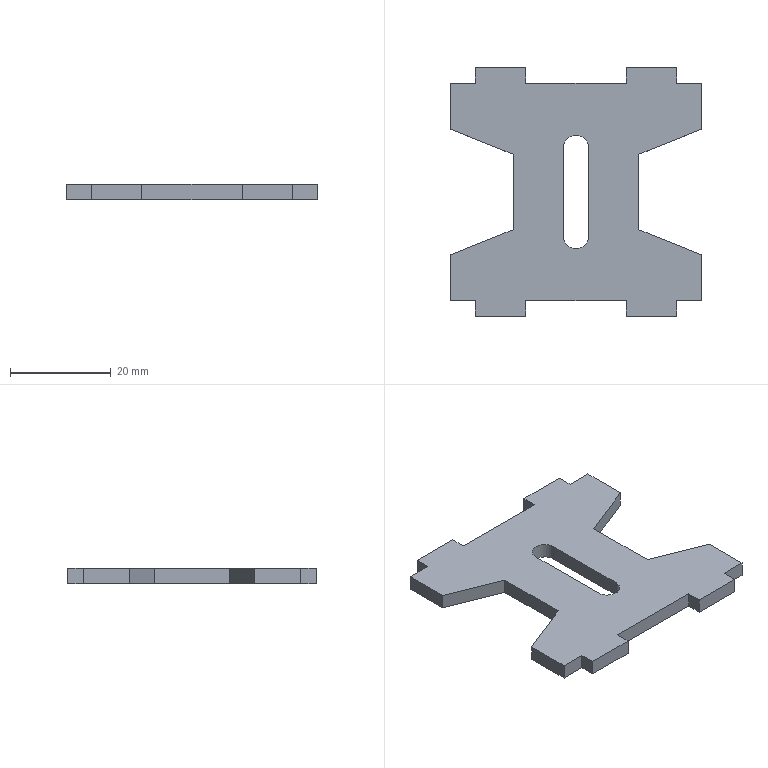Part | SolidWorks | features Extrusion 1 | 1 solid | 34 faces | box 50 x 49.3 x 3 mm | volume 5034 mm3 | plane 32 | cylinder 2 | commonest cylinder face diameters 5 x2
STEP:
#1=CARTESIAN_POINT('',(-25.609,-21.769,3.));
#2=VERTEX_POINT('',#1);
#3=CARTESIAN_POINT('',(-25.609,-12.619,3.));
#4=VERTEX_POINT('',#3);
#5=CARTESIAN_POINT('',(-25.609,-21.769,3.));
#6=DIRECTION('',(0.,1.,0.));
#7=VECTOR('',#6,1000.);
#8=LINE('',#5,#7);
#9=EDGE_CURVE('',#2,#4,#8,.T.);
#10=ORIENTED_EDGE('',*,*,#9,.F.);
#11=CARTESIAN_POINT('',(-20.609,-21.769,3.));
#12=VERTEX_POINT('',#11);
#13=CARTESIAN_POINT('',(-25.609,-21.769,3.));
#14=DIRECTION('',(1.,0.,0.));
#15=VECTOR('',#14,1000.);
#16=LINE('',#13,#15);
#17=EDGE_CURVE('',#2,#12,#16,.T.);
#18=ORIENTED_EDGE('',*,*,#17,.T.);
#19=CARTESIAN_POINT('',(-20.609,-24.769,3.));
#20=VERTEX_POINT('',#19);
#21=CARTESIAN_POINT('',(-20.609,-21.769,3.));
#22=DIRECTION('',(0.,-1.,0.));
#23=VECTOR('',#22,1000.);
#24=LINE('',#21,#23);
#25=EDGE_CURVE('',#12,#20,#24,.T.);
#26=ORIENTED_EDGE('',*,*,#25,.T.);
#27=CARTESIAN_POINT('',(-10.609,-24.769,3.));
#28=VERTEX_POINT('',#27);
#29=CARTESIAN_POINT('',(-20.609,-24.769,3.));
#30=DIRECTION('',(1.,0.,0.));
#31=VECTOR('',#30,1000.);
#32=LINE('',#29,#31);
#33=EDGE_CURVE('',#20,#28,#32,.T.);
#34=ORIENTED_EDGE('',*,*,#33,.T.);
#35=CARTESIAN_POINT('',(-10.609,-21.769,3.));
#36=VERTEX_POINT('',#35);
#37=CARTESIAN_POINT('',(-10.609,-24.769,3.));
#38=DIRECTION('',(0.,1.,0.));
#39=VECTOR('',#38,1000.);
#40=LINE('',#37,#39);
#41=EDGE_CURVE('',#28,#36,#40,.T.);
#42=ORIENTED_EDGE('',*,*,#41,.T.);
#43=CARTESIAN_POINT('',(9.391,-21.769,3.));
#44=VERTEX_POINT('',#43);
#45=CARTESIAN_POINT('',(-10.609,-21.769,3.));
#46=DIRECTION('',(1.,0.,0.));
#47=VECTOR('',#46,1000.);
#48=LINE('',#45,#47);
#49=EDGE_CURVE('',#36,#44,#48,.T.);
#50=ORIENTED_EDGE('',*,*,#49,.T.);
#51=CARTESIAN_POINT('',(9.391,-24.769,3.));
#52=VERTEX_POINT('',#51);
#53=CARTESIAN_POINT('',(9.391,-24.769,3.));
#54=DIRECTION('',(0.,1.,0.));
#55=VECTOR('',#54,1000.);
#56=LINE('',#53,#55);
#57=EDGE_CURVE('',#52,#44,#56,.T.);
#58=ORIENTED_EDGE('',*,*,#57,.F.);
#59=CARTESIAN_POINT('',(19.391,-24.769,3.));
#60=VERTEX_POINT('',#59);
#61=CARTESIAN_POINT('',(19.391,-24.769,3.));
#62=DIRECTION('',(-1.,0.,0.));
#63=VECTOR('',#62,1000.);
#64=LINE('',#61,#63);
#65=EDGE_CURVE('',#60,#52,#64,.T.);
#66=ORIENTED_EDGE('',*,*,#65,.F.);
#67=CARTESIAN_POINT('',(19.391,-21.769,3.));
#68=VERTEX_POINT('',#67);
#69=CARTESIAN_POINT('',(19.391,-21.769,3.));
#70=DIRECTION('',(0.,-1.,0.));
#71=VECTOR('',#70,1000.);
#72=LINE('',#69,#71);
#73=EDGE_CURVE('',#68,#60,#72,.T.);
#74=ORIENTED_EDGE('',*,*,#73,.F.);
#75=CARTESIAN_POINT('',(24.391,-21.769,3.));
#76=VERTEX_POINT('',#75);
#77=CARTESIAN_POINT('',(19.391,-21.769,3.));
#78=DIRECTION('',(1.,0.,0.));
#79=VECTOR('',#78,1000.);
#80=LINE('',#77,#79);
#81=EDGE_CURVE('',#68,#76,#80,.T.);
#82=ORIENTED_EDGE('',*,*,#81,.T.);
#83=CARTESIAN_POINT('',(24.391,-12.619,3.));
#84=VERTEX_POINT('',#83);
#85=CARTESIAN_POINT('',(24.391,-21.769,3.));
#86=DIRECTION('',(0.,1.,0.));
#87=VECTOR('',#86,1000.);
#88=LINE('',#85,#87);
#89=EDGE_CURVE('',#76,#84,#88,.T.);
#90=ORIENTED_EDGE('',*,*,#89,.T.);
#91=CARTESIAN_POINT('',(11.891,-7.619,3.));
#92=VERTEX_POINT('',#91);
#93=CARTESIAN_POINT('',(11.891,-7.619,3.));
#94=DIRECTION('',(0.9285,-0.3714,0.));
#95=VECTOR('',#94,1000.);
#96=LINE('',#93,#95);
#97=EDGE_CURVE('',#92,#84,#96,.T.);
#98=ORIENTED_EDGE('',*,*,#97,.F.);
#99=CARTESIAN_POINT('',(11.891,7.381,3.));
#100=VERTEX_POINT('',#99);
#101=CARTESIAN_POINT('',(11.891,7.381,3.));
#102=DIRECTION('',(0.,-1.,0.));
#103=VECTOR('',#102,1000.);
#104=LINE('',#101,#103);
#105=EDGE_CURVE('',#100,#92,#104,.T.);
#106=ORIENTED_EDGE('',*,*,#105,.F.);
#107=CARTESIAN_POINT('',(24.391,12.381,3.));
#108=VERTEX_POINT('',#107);
#109=CARTESIAN_POINT('',(24.391,12.381,3.));
#110=DIRECTION('',(-0.9285,-0.3714,0.));
#111=VECTOR('',#110,1000.);
#112=LINE('',#109,#111);
#113=EDGE_CURVE('',#108,#100,#112,.T.);
#114=ORIENTED_EDGE('',*,*,#113,.F.);
#115=CARTESIAN_POINT('',(24.391,21.531,3.));
#116=VERTEX_POINT('',#115);
#117=CARTESIAN_POINT('',(24.391,12.381,3.));
#118=DIRECTION('',(0.,1.,0.));
#119=VECTOR('',#118,1000.);
#120=LINE('',#117,#119);
#121=EDGE_CURVE('',#108,#116,#120,.T.);
#122=ORIENTED_EDGE('',*,*,#121,.T.);
#123=CARTESIAN_POINT('',(19.391,21.531,3.));
#124=VERTEX_POINT('',#123);
#125=CARTESIAN_POINT('',(19.391,21.531,3.));
#126=DIRECTION('',(1.,0.,0.));
#127=VECTOR('',#126,1000.);
#128=LINE('',#125,#127);
#129=EDGE_CURVE('',#124,#116,#128,.T.);
#130=ORIENTED_EDGE('',*,*,#129,.F.);
#131=CARTESIAN_POINT('',(19.391,24.531,3.));
#132=VERTEX_POINT('',#131);
#133=CARTESIAN_POINT('',(19.391,21.531,3.));
#134=DIRECTION('',(0.,1.,0.));
#135=VECTOR('',#134,1000.);
#136=LINE('',#133,#135);
#137=EDGE_CURVE('',#124,#132,#136,.T.);
#138=ORIENTED_EDGE('',*,*,#137,.T.);
#139=CARTESIAN_POINT('',(9.391,24.531,3.));
#140=VERTEX_POINT('',#139);
#141=CARTESIAN_POINT('',(19.391,24.531,3.));
#142=DIRECTION('',(-1.,0.,0.));
#143=VECTOR('',#142,1000.);
#144=LINE('',#141,#143);
#145=EDGE_CURVE('',#132,#140,#144,.T.);
#146=ORIENTED_EDGE('',*,*,#145,.T.);
#147=CARTESIAN_POINT('',(9.391,21.531,3.));
#148=VERTEX_POINT('',#147);
#149=CARTESIAN_POINT('',(9.391,24.531,3.));
#150=DIRECTION('',(0.,-1.,0.));
#151=VECTOR('',#150,1000.);
#152=LINE('',#149,#151);
#153=EDGE_CURVE('',#140,#148,#152,.T.);
#154=ORIENTED_EDGE('',*,*,#153,.T.);
#155=CARTESIAN_POINT('',(-10.609,21.531,3.));
#156=VERTEX_POINT('',#155);
#157=CARTESIAN_POINT('',(-10.609,21.531,3.));
#158=DIRECTION('',(1.,0.,0.));
#159=VECTOR('',#158,1000.);
#160=LINE('',#157,#159);
#161=EDGE_CURVE('',#156,#148,#160,.T.);
#162=ORIENTED_EDGE('',*,*,#161,.F.);
#163=CARTESIAN_POINT('',(-10.609,24.531,3.));
#164=VERTEX_POINT('',#163);
#165=CARTESIAN_POINT('',(-10.609,24.531,3.));
#166=DIRECTION('',(0.,-1.,0.));
#167=VECTOR('',#166,1000.);
#168=LINE('',#165,#167);
#169=EDGE_CURVE('',#164,#156,#168,.T.);
#170=ORIENTED_EDGE('',*,*,#169,.F.);
#171=CARTESIAN_POINT('',(-20.609,24.531,3.));
#172=VERTEX_POINT('',#171);
#173=CARTESIAN_POINT('',(-20.609,24.531,3.));
#174=DIRECTION('',(1.,0.,0.));
#175=VECTOR('',#174,1000.);
#176=LINE('',#173,#175);
#177=EDGE_CURVE('',#172,#164,#176,.T.);
#178=ORIENTED_EDGE('',*,*,#177,.F.);
#179=CARTESIAN_POINT('',(-20.609,21.531,3.));
#180=VERTEX_POINT('',#179);
#181=CARTESIAN_POINT('',(-20.609,21.531,3.));
#182=DIRECTION('',(0.,1.,0.));
#183=VECTOR('',#182,1000.);
#184=LINE('',#181,#183);
#185=EDGE_CURVE('',#180,#172,#184,.T.);
#186=ORIENTED_EDGE('',*,*,#185,.F.);
#187=CARTESIAN_POINT('',(-25.609,21.531,3.));
#188=VERTEX_POINT('',#187);
#189=CARTESIAN_POINT('',(-25.609,21.531,3.));
#190=DIRECTION('',(1.,0.,0.));
#191=VECTOR('',#190,1000.);
#192=LINE('',#189,#191);
#193=EDGE_CURVE('',#188,#180,#192,.T.);
#194=ORIENTED_EDGE('',*,*,#193,.F.);
#195=CARTESIAN_POINT('',(-25.609,12.381,3.));
#196=VERTEX_POINT('',#195);
#197=CARTESIAN_POINT('',(-25.609,12.381,3.));
#198=DIRECTION('',(0.,1.,0.));
#199=VECTOR('',#198,1000.);
#200=LINE('',#197,#199);
#201=EDGE_CURVE('',#196,#188,#200,.T.);
#202=ORIENTED_EDGE('',*,*,#201,.F.);
#203=CARTESIAN_POINT('',(-13.109,7.381,3.));
#204=VERTEX_POINT('',#203);
#205=CARTESIAN_POINT('',(-25.609,12.381,3.));
#206=DIRECTION('',(0.9285,-0.3714,0.));
#207=VECTOR('',#206,1000.);
#208=LINE('',#205,#207);
#209=EDGE_CURVE('',#196,#204,#208,.T.);
#210=ORIENTED_EDGE('',*,*,#209,.T.);
#211=CARTESIAN_POINT('',(-13.109,-7.619,3.));
#212=VERTEX_POINT('',#211);
#213=CARTESIAN_POINT('',(-13.109,7.381,3.));
#214=DIRECTION('',(0.,-1.,0.));
#215=VECTOR('',#214,1000.);
#216=LINE('',#213,#215);
#217=EDGE_CURVE('',#204,#212,#216,.T.);
#218=ORIENTED_EDGE('',*,*,#217,.T.);
#219=CARTESIAN_POINT('',(-13.109,-7.619,3.));
#220=DIRECTION('',(-0.9285,-0.3714,0.));
#221=VECTOR('',#220,1000.);
#222=LINE('',#219,#221);
#223=EDGE_CURVE('',#212,#4,#222,.T.);
#224=ORIENTED_EDGE('',*,*,#223,.T.);
#225=EDGE_LOOP('',(#10,#18,#26,#34,#42,#50,#58,#66,#74,#82,#90,#98,#106,#114,#122,#130,#138,#146,#154,#162,#170,#178,#186,#194,#202,#210,#218,#224));
#226=FACE_OUTER_BOUND('',#225,.T.);
#227=CARTESIAN_POINT('',(1.891,8.631,3.));
#228=VERTEX_POINT('',#227);
#229=CARTESIAN_POINT('',(-3.109,8.631,3.));
#230=VERTEX_POINT('',#229);
#231=CARTESIAN_POINT('',(-0.6092,8.631,3.));
#232=DIRECTION('',(0.,0.,1.));
#233=DIRECTION('',(1.,0.,0.));
#234=AXIS2_PLACEMENT_3D('',#231,#232,#233);
#235=CIRCLE('',#234,2.5);
#236=EDGE_CURVE('',#228,#230,#235,.T.);
#237=ORIENTED_EDGE('',*,*,#236,.F.);
#238=CARTESIAN_POINT('',(1.891,-8.869,3.));
#239=VERTEX_POINT('',#238);
#240=CARTESIAN_POINT('',(1.891,8.631,3.));
#241=DIRECTION('',(0.,-1.,0.));
#242=VECTOR('',#241,1000.);
#243=LINE('',#240,#242);
#244=EDGE_CURVE('',#228,#239,#243,.T.);
#245=ORIENTED_EDGE('',*,*,#244,.T.);
#246=CARTESIAN_POINT('',(-3.109,-8.869,3.));
#247=VERTEX_POINT('',#246);
#248=CARTESIAN_POINT('',(-0.6092,-8.869,3.));
#249=DIRECTION('',(0.,0.,1.));
#250=DIRECTION('',(1.,0.,0.));
#251=AXIS2_PLACEMENT_3D('',#248,#249,#250);
#252=CIRCLE('',#251,2.5);
#253=EDGE_CURVE('',#247,#239,#252,.T.);
#254=ORIENTED_EDGE('',*,*,#253,.F.);
#255=CARTESIAN_POINT('',(-3.109,8.631,3.));
#256=DIRECTION('',(0.,-1.,0.));
#257=VECTOR('',#256,1000.);
#258=LINE('',#255,#257);
#259=EDGE_CURVE('',#230,#247,#258,.T.);
#260=ORIENTED_EDGE('',*,*,#259,.F.);
#261=EDGE_LOOP('',(#237,#245,#254,#260));
#262=FACE_BOUND('',#261,.T.);
#263=CARTESIAN_POINT('',(0.,0.,3.));
#264=DIRECTION('',(0.,0.,-1.));
#265=DIRECTION('',(-1.,0.,0.));
#266=AXIS2_PLACEMENT_3D('',#263,#264,#265);
#267=PLANE('',#266);
#268=ADVANCED_FACE('',(#226,#262),#267,.F.);
#269=CARTESIAN_POINT('',(-25.609,-21.769,0.));
#270=VERTEX_POINT('',#269);
#271=CARTESIAN_POINT('',(-25.609,-12.619,0.));
#272=VERTEX_POINT('',#271);
#273=CARTESIAN_POINT('',(-25.609,-21.769,0.));
#274=DIRECTION('',(0.,1.,0.));
#275=VECTOR('',#274,1000.);
#276=LINE('',#273,#275);
#277=EDGE_CURVE('',#270,#272,#276,.T.);
#278=ORIENTED_EDGE('',*,*,#277,.T.);
#279=CARTESIAN_POINT('',(-13.109,-7.619,0.));
#280=VERTEX_POINT('',#279);
#281=CARTESIAN_POINT('',(-13.109,-7.619,0.));
#282=DIRECTION('',(-0.9285,-0.3714,0.));
#283=VECTOR('',#282,1000.);
#284=LINE('',#281,#283);
#285=EDGE_CURVE('',#280,#272,#284,.T.);
#286=ORIENTED_EDGE('',*,*,#285,.F.);
#287=CARTESIAN_POINT('',(-13.109,7.381,0.));
#288=VERTEX_POINT('',#287);
#289=CARTESIAN_POINT('',(-13.109,7.381,0.));
#290=DIRECTION('',(0.,-1.,0.));
#291=VECTOR('',#290,1000.);
#292=LINE('',#289,#291);
#293=EDGE_CURVE('',#288,#280,#292,.T.);
#294=ORIENTED_EDGE('',*,*,#293,.F.);
#295=CARTESIAN_POINT('',(-25.609,12.381,0.));
#296=VERTEX_POINT('',#295);
#297=CARTESIAN_POINT('',(-25.609,12.381,0.));
#298=DIRECTION('',(0.9285,-0.3714,0.));
#299=VECTOR('',#298,1000.);
#300=LINE('',#297,#299);
#301=EDGE_CURVE('',#296,#288,#300,.T.);
#302=ORIENTED_EDGE('',*,*,#301,.F.);
#303=CARTESIAN_POINT('',(-25.609,21.531,0.));
#304=VERTEX_POINT('',#303);
#305=CARTESIAN_POINT('',(-25.609,12.381,0.));
#306=DIRECTION('',(0.,1.,0.));
#307=VECTOR('',#306,1000.);
#308=LINE('',#305,#307);
#309=EDGE_CURVE('',#296,#304,#308,.T.);
#310=ORIENTED_EDGE('',*,*,#309,.T.);
#311=CARTESIAN_POINT('',(-20.609,21.531,0.));
#312=VERTEX_POINT('',#311);
#313=CARTESIAN_POINT('',(-25.609,21.531,0.));
#314=DIRECTION('',(1.,0.,0.));
#315=VECTOR('',#314,1000.);
#316=LINE('',#313,#315);
#317=EDGE_CURVE('',#304,#312,#316,.T.);
#318=ORIENTED_EDGE('',*,*,#317,.T.);
#319=CARTESIAN_POINT('',(-20.609,24.531,0.));
#320=VERTEX_POINT('',#319);
#321=CARTESIAN_POINT('',(-20.609,21.531,0.));
#322=DIRECTION('',(0.,1.,0.));
#323=VECTOR('',#322,1000.);
#324=LINE('',#321,#323);
#325=EDGE_CURVE('',#312,#320,#324,.T.);
#326=ORIENTED_EDGE('',*,*,#325,.T.);
#327=CARTESIAN_POINT('',(-10.609,24.531,0.));
#328=VERTEX_POINT('',#327);
#329=CARTESIAN_POINT('',(-20.609,24.531,0.));
#330=DIRECTION('',(1.,0.,0.));
#331=VECTOR('',#330,1000.);
#332=LINE('',#329,#331);
#333=EDGE_CURVE('',#320,#328,#332,.T.);
#334=ORIENTED_EDGE('',*,*,#333,.T.);
#335=CARTESIAN_POINT('',(-10.609,21.531,0.));
#336=VERTEX_POINT('',#335);
#337=CARTESIAN_POINT('',(-10.609,24.531,0.));
#338=DIRECTION('',(0.,-1.,0.));
#339=VECTOR('',#338,1000.);
#340=LINE('',#337,#339);
#341=EDGE_CURVE('',#328,#336,#340,.T.);
#342=ORIENTED_EDGE('',*,*,#341,.T.);
#343=CARTESIAN_POINT('',(9.391,21.531,0.));
#344=VERTEX_POINT('',#343);
#345=CARTESIAN_POINT('',(-10.609,21.531,0.));
#346=DIRECTION('',(1.,0.,0.));
#347=VECTOR('',#346,1000.);
#348=LINE('',#345,#347);
#349=EDGE_CURVE('',#336,#344,#348,.T.);
#350=ORIENTED_EDGE('',*,*,#349,.T.);
#351=CARTESIAN_POINT('',(9.391,24.531,0.));
#352=VERTEX_POINT('',#351);
#353=CARTESIAN_POINT('',(9.391,24.531,0.));
#354=DIRECTION('',(0.,-1.,0.));
#355=VECTOR('',#354,1000.);
#356=LINE('',#353,#355);
#357=EDGE_CURVE('',#352,#344,#356,.T.);
#358=ORIENTED_EDGE('',*,*,#357,.F.);
#359=CARTESIAN_POINT('',(19.391,24.531,0.));
#360=VERTEX_POINT('',#359);
#361=CARTESIAN_POINT('',(19.391,24.531,0.));
#362=DIRECTION('',(-1.,0.,0.));
#363=VECTOR('',#362,1000.);
#364=LINE('',#361,#363);
#365=EDGE_CURVE('',#360,#352,#364,.T.);
#366=ORIENTED_EDGE('',*,*,#365,.F.);
#367=CARTESIAN_POINT('',(19.391,21.531,0.));
#368=VERTEX_POINT('',#367);
#369=CARTESIAN_POINT('',(19.391,21.531,0.));
#370=DIRECTION('',(0.,1.,0.));
#371=VECTOR('',#370,1000.);
#372=LINE('',#369,#371);
#373=EDGE_CURVE('',#368,#360,#372,.T.);
#374=ORIENTED_EDGE('',*,*,#373,.F.);
#375=CARTESIAN_POINT('',(24.391,21.531,0.));
#376=VERTEX_POINT('',#375);
#377=CARTESIAN_POINT('',(19.391,21.531,0.));
#378=DIRECTION('',(1.,0.,0.));
#379=VECTOR('',#378,1000.);
#380=LINE('',#377,#379);
#381=EDGE_CURVE('',#368,#376,#380,.T.);
#382=ORIENTED_EDGE('',*,*,#381,.T.);
#383=CARTESIAN_POINT('',(24.391,12.381,0.));
#384=VERTEX_POINT('',#383);
#385=CARTESIAN_POINT('',(24.391,12.381,0.));
#386=DIRECTION('',(0.,1.,0.));
#387=VECTOR('',#386,1000.);
#388=LINE('',#385,#387);
#389=EDGE_CURVE('',#384,#376,#388,.T.);
#390=ORIENTED_EDGE('',*,*,#389,.F.);
#391=CARTESIAN_POINT('',(11.891,7.381,0.));
#392=VERTEX_POINT('',#391);
#393=CARTESIAN_POINT('',(24.391,12.381,0.));
#394=DIRECTION('',(-0.9285,-0.3714,0.));
#395=VECTOR('',#394,1000.);
#396=LINE('',#393,#395);
#397=EDGE_CURVE('',#384,#392,#396,.T.);
#398=ORIENTED_EDGE('',*,*,#397,.T.);
#399=CARTESIAN_POINT('',(11.891,-7.619,0.));
#400=VERTEX_POINT('',#399);
#401=CARTESIAN_POINT('',(11.891,7.381,0.));
#402=DIRECTION('',(0.,-1.,0.));
#403=VECTOR('',#402,1000.);
#404=LINE('',#401,#403);
#405=EDGE_CURVE('',#392,#400,#404,.T.);
#406=ORIENTED_EDGE('',*,*,#405,.T.);
#407=CARTESIAN_POINT('',(24.391,-12.619,0.));
#408=VERTEX_POINT('',#407);
#409=CARTESIAN_POINT('',(11.891,-7.619,0.));
#410=DIRECTION('',(0.9285,-0.3714,0.));
#411=VECTOR('',#410,1000.);
#412=LINE('',#409,#411);
#413=EDGE_CURVE('',#400,#408,#412,.T.);
#414=ORIENTED_EDGE('',*,*,#413,.T.);
#415=CARTESIAN_POINT('',(24.391,-21.769,0.));
#416=VERTEX_POINT('',#415);
#417=CARTESIAN_POINT('',(24.391,-21.769,0.));
#418=DIRECTION('',(0.,1.,0.));
#419=VECTOR('',#418,1000.);
#420=LINE('',#417,#419);
#421=EDGE_CURVE('',#416,#408,#420,.T.);
#422=ORIENTED_EDGE('',*,*,#421,.F.);
#423=CARTESIAN_POINT('',(19.391,-21.769,0.));
#424=VERTEX_POINT('',#423);
#425=CARTESIAN_POINT('',(19.391,-21.769,0.));
#426=DIRECTION('',(1.,0.,0.));
#427=VECTOR('',#426,1000.);
#428=LINE('',#425,#427);
#429=EDGE_CURVE('',#424,#416,#428,.T.);
#430=ORIENTED_EDGE('',*,*,#429,.F.);
#431=CARTESIAN_POINT('',(19.391,-24.769,0.));
#432=VERTEX_POINT('',#431);
#433=CARTESIAN_POINT('',(19.391,-21.769,0.));
#434=DIRECTION('',(0.,-1.,0.));
#435=VECTOR('',#434,1000.);
#436=LINE('',#433,#435);
#437=EDGE_CURVE('',#424,#432,#436,.T.);
#438=ORIENTED_EDGE('',*,*,#437,.T.);
#439=CARTESIAN_POINT('',(9.391,-24.769,0.));
#440=VERTEX_POINT('',#439);
#441=CARTESIAN_POINT('',(19.391,-24.769,0.));
#442=DIRECTION('',(-1.,0.,0.));
#443=VECTOR('',#442,1000.);
#444=LINE('',#441,#443);
#445=EDGE_CURVE('',#432,#440,#444,.T.);
#446=ORIENTED_EDGE('',*,*,#445,.T.);
#447=CARTESIAN_POINT('',(9.391,-21.769,0.));
#448=VERTEX_POINT('',#447);
#449=CARTESIAN_POINT('',(9.391,-24.769,0.));
#450=DIRECTION('',(0.,1.,0.));
#451=VECTOR('',#450,1000.);
#452=LINE('',#449,#451);
#453=EDGE_CURVE('',#440,#448,#452,.T.);
#454=ORIENTED_EDGE('',*,*,#453,.T.);
#455=CARTESIAN_POINT('',(-10.609,-21.769,0.));
#456=VERTEX_POINT('',#455);
#457=CARTESIAN_POINT('',(-10.609,-21.769,0.));
#458=DIRECTION('',(1.,0.,0.));
#459=VECTOR('',#458,1000.);
#460=LINE('',#457,#459);
#461=EDGE_CURVE('',#456,#448,#460,.T.);
#462=ORIENTED_EDGE('',*,*,#461,.F.);
#463=CARTESIAN_POINT('',(-10.609,-24.769,0.));
#464=VERTEX_POINT('',#463);
#465=CARTESIAN_POINT('',(-10.609,-24.769,0.));
#466=DIRECTION('',(0.,1.,0.));
#467=VECTOR('',#466,1000.);
#468=LINE('',#465,#467);
#469=EDGE_CURVE('',#464,#456,#468,.T.);
#470=ORIENTED_EDGE('',*,*,#469,.F.);
#471=CARTESIAN_POINT('',(-20.609,-24.769,0.));
#472=VERTEX_POINT('',#471);
#473=CARTESIAN_POINT('',(-20.609,-24.769,0.));
#474=DIRECTION('',(1.,0.,0.));
#475=VECTOR('',#474,1000.);
#476=LINE('',#473,#475);
#477=EDGE_CURVE('',#472,#464,#476,.T.);
#478=ORIENTED_EDGE('',*,*,#477,.F.);
#479=CARTESIAN_POINT('',(-20.609,-21.769,0.));
#480=VERTEX_POINT('',#479);
#481=CARTESIAN_POINT('',(-20.609,-21.769,0.));
#482=DIRECTION('',(0.,-1.,0.));
#483=VECTOR('',#482,1000.);
#484=LINE('',#481,#483);
#485=EDGE_CURVE('',#480,#472,#484,.T.);
#486=ORIENTED_EDGE('',*,*,#485,.F.);
#487=CARTESIAN_POINT('',(-25.609,-21.769,0.));
#488=DIRECTION('',(1.,0.,0.));
#489=VECTOR('',#488,1000.);
#490=LINE('',#487,#489);
#491=EDGE_CURVE('',#270,#480,#490,.T.);
#492=ORIENTED_EDGE('',*,*,#491,.F.);
#493=EDGE_LOOP('',(#278,#286,#294,#302,#310,#318,#326,#334,#342,#350,#358,#366,#374,#382,#390,#398,#406,#414,#422,#430,#438,#446,#454,#462,#470,#478,#486,#492));
#494=FACE_OUTER_BOUND('',#493,.T.);
#495=CARTESIAN_POINT('',(1.891,8.631,0.));
#496=VERTEX_POINT('',#495);
#497=CARTESIAN_POINT('',(1.891,-8.869,0.));
#498=VERTEX_POINT('',#497);
#499=CARTESIAN_POINT('',(1.891,8.631,0.));
#500=DIRECTION('',(0.,-1.,0.));
#501=VECTOR('',#500,1000.);
#502=LINE('',#499,#501);
#503=EDGE_CURVE('',#496,#498,#502,.T.);
#504=ORIENTED_EDGE('',*,*,#503,.F.);
#505=CARTESIAN_POINT('',(-3.109,8.631,0.));
#506=VERTEX_POINT('',#505);
#507=CARTESIAN_POINT('',(-0.6092,8.631,0.));
#508=DIRECTION('',(0.,0.,1.));
#509=DIRECTION('',(1.,0.,0.));
#510=AXIS2_PLACEMENT_3D('',#507,#508,#509);
#511=CIRCLE('',#510,2.5);
#512=EDGE_CURVE('',#496,#506,#511,.T.);
#513=ORIENTED_EDGE('',*,*,#512,.T.);
#514=CARTESIAN_POINT('',(-3.109,-8.869,0.));
#515=VERTEX_POINT('',#514);
#516=CARTESIAN_POINT('',(-3.109,8.631,0.));
#517=DIRECTION('',(0.,-1.,0.));
#518=VECTOR('',#517,1000.);
#519=LINE('',#516,#518);
#520=EDGE_CURVE('',#506,#515,#519,.T.);
#521=ORIENTED_EDGE('',*,*,#520,.T.);
#522=CARTESIAN_POINT('',(-0.6092,-8.869,0.));
#523=DIRECTION('',(0.,0.,1.));
#524=DIRECTION('',(1.,0.,0.));
#525=AXIS2_PLACEMENT_3D('',#522,#523,#524);
#526=CIRCLE('',#525,2.5);
#527=EDGE_CURVE('',#515,#498,#526,.T.);
#528=ORIENTED_EDGE('',*,*,#527,.T.);
#529=EDGE_LOOP('',(#504,#513,#521,#528));
#530=FACE_BOUND('',#529,.T.);
#531=CARTESIAN_POINT('',(0.,0.,0.));
#532=DIRECTION('',(0.,0.,-1.));
#533=DIRECTION('',(-1.,0.,0.));
#534=AXIS2_PLACEMENT_3D('',#531,#532,#533);
#535=PLANE('',#534);
#536=ADVANCED_FACE('',(#494,#530),#535,.T.);
#537=ORIENTED_EDGE('',*,*,#277,.F.);
#538=CARTESIAN_POINT('',(-25.609,-21.769,3.));
#539=DIRECTION('',(0.,0.,-1.));
#540=VECTOR('',#539,1000.);
#541=LINE('',#538,#540);
#542=EDGE_CURVE('',#2,#270,#541,.T.);
#543=ORIENTED_EDGE('',*,*,#542,.F.);
#544=ORIENTED_EDGE('',*,*,#9,.T.);
#545=CARTESIAN_POINT('',(-25.609,-12.619,3.));
#546=DIRECTION('',(0.,0.,-1.));
#547=VECTOR('',#546,1000.);
#548=LINE('',#545,#547);
#549=EDGE_CURVE('',#4,#272,#548,.T.);
#550=ORIENTED_EDGE('',*,*,#549,.T.);
#551=EDGE_LOOP('',(#537,#543,#544,#550));
#552=FACE_OUTER_BOUND('',#551,.T.);
#553=CARTESIAN_POINT('',(-25.609,-21.769,3.));
#554=DIRECTION('',(-1.,0.,0.));
#555=DIRECTION('',(0.,0.,1.));
#556=AXIS2_PLACEMENT_3D('',#553,#554,#555);
#557=PLANE('',#556);
#558=ADVANCED_FACE('',(#552),#557,.T.);
#559=ORIENTED_EDGE('',*,*,#491,.T.);
#560=CARTESIAN_POINT('',(-20.609,-21.769,3.));
#561=DIRECTION('',(0.,0.,-1.));
#562=VECTOR('',#561,1000.);
#563=LINE('',#560,#562);
#564=EDGE_CURVE('',#12,#480,#563,.T.);
#565=ORIENTED_EDGE('',*,*,#564,.F.);
#566=ORIENTED_EDGE('',*,*,#17,.F.);
#567=ORIENTED_EDGE('',*,*,#542,.T.);
#568=EDGE_LOOP('',(#559,#565,#566,#567));
#569=FACE_OUTER_BOUND('',#568,.T.);
#570=CARTESIAN_POINT('',(-25.609,-21.769,3.));
#571=DIRECTION('',(0.,1.,0.));
#572=DIRECTION('',(0.,0.,1.));
#573=AXIS2_PLACEMENT_3D('',#570,#571,#572);
#574=PLANE('',#573);
#575=ADVANCED_FACE('',(#569),#574,.F.);
#576=ORIENTED_EDGE('',*,*,#485,.T.);
#577=CARTESIAN_POINT('',(-20.609,-24.769,3.));
#578=DIRECTION('',(0.,0.,-1.));
#579=VECTOR('',#578,1000.);
#580=LINE('',#577,#579);
#581=EDGE_CURVE('',#20,#472,#580,.T.);
#582=ORIENTED_EDGE('',*,*,#581,.F.);
#583=ORIENTED_EDGE('',*,*,#25,.F.);
#584=ORIENTED_EDGE('',*,*,#564,.T.);
#585=EDGE_LOOP('',(#576,#582,#583,#584));
#586=FACE_OUTER_BOUND('',#585,.T.);
#587=CARTESIAN_POINT('',(-20.609,-21.769,3.));
#588=DIRECTION('',(1.,0.,0.));
#589=DIRECTION('',(0.,0.,-1.));
#590=AXIS2_PLACEMENT_3D('',#587,#588,#589);
#591=PLANE('',#590);
#592=ADVANCED_FACE('',(#586),#591,.F.);
#593=ORIENTED_EDGE('',*,*,#477,.T.);
#594=CARTESIAN_POINT('',(-10.609,-24.769,3.));
#595=DIRECTION('',(0.,0.,-1.));
#596=VECTOR('',#595,1000.);
#597=LINE('',#594,#596);
#598=EDGE_CURVE('',#28,#464,#597,.T.);
#599=ORIENTED_EDGE('',*,*,#598,.F.);
#600=ORIENTED_EDGE('',*,*,#33,.F.);
#601=ORIENTED_EDGE('',*,*,#581,.T.);
#602=EDGE_LOOP('',(#593,#599,#600,#601));
#603=FACE_OUTER_BOUND('',#602,.T.);
#604=CARTESIAN_POINT('',(-20.609,-24.769,3.));
#605=DIRECTION('',(0.,1.,0.));
#606=DIRECTION('',(-1.,0.,0.));
#607=AXIS2_PLACEMENT_3D('',#604,#605,#606);
#608=PLANE('',#607);
#609=ADVANCED_FACE('',(#603),#608,.F.);
#610=ORIENTED_EDGE('',*,*,#469,.T.);
#611=CARTESIAN_POINT('',(-10.609,-21.769,3.));
#612=DIRECTION('',(0.,0.,-1.));
#613=VECTOR('',#612,1000.);
#614=LINE('',#611,#613);
#615=EDGE_CURVE('',#36,#456,#614,.T.);
#616=ORIENTED_EDGE('',*,*,#615,.F.);
#617=ORIENTED_EDGE('',*,*,#41,.F.);
#618=ORIENTED_EDGE('',*,*,#598,.T.);
#619=EDGE_LOOP('',(#610,#616,#617,#618));
#620=FACE_OUTER_BOUND('',#619,.T.);
#621=CARTESIAN_POINT('',(-10.609,-24.769,3.));
#622=DIRECTION('',(-1.,0.,0.));
#623=DIRECTION('',(0.,-1.,0.));
#624=AXIS2_PLACEMENT_3D('',#621,#622,#623);
#625=PLANE('',#624);
#626=ADVANCED_FACE('',(#620),#625,.F.);
#627=ORIENTED_EDGE('',*,*,#461,.T.);
#628=CARTESIAN_POINT('',(9.391,-21.769,3.));
#629=DIRECTION('',(0.,0.,-1.));
#630=VECTOR('',#629,1000.);
#631=LINE('',#628,#630);
#632=EDGE_CURVE('',#44,#448,#631,.T.);
#633=ORIENTED_EDGE('',*,*,#632,.F.);
#634=ORIENTED_EDGE('',*,*,#49,.F.);
#635=ORIENTED_EDGE('',*,*,#615,.T.);
#636=EDGE_LOOP('',(#627,#633,#634,#635));
#637=FACE_OUTER_BOUND('',#636,.T.);
#638=CARTESIAN_POINT('',(-10.609,-21.769,3.));
#639=DIRECTION('',(0.,1.,0.));
#640=DIRECTION('',(0.,0.,1.));
#641=AXIS2_PLACEMENT_3D('',#638,#639,#640);
#642=PLANE('',#641);
#643=ADVANCED_FACE('',(#637),#642,.F.);
#644=ORIENTED_EDGE('',*,*,#453,.F.);
#645=CARTESIAN_POINT('',(9.391,-24.769,3.));
#646=DIRECTION('',(0.,0.,-1.));
#647=VECTOR('',#646,1000.);
#648=LINE('',#645,#647);
#649=EDGE_CURVE('',#52,#440,#648,.T.);
#650=ORIENTED_EDGE('',*,*,#649,.F.);
#651=ORIENTED_EDGE('',*,*,#57,.T.);
#652=ORIENTED_EDGE('',*,*,#632,.T.);
#653=EDGE_LOOP('',(#644,#650,#651,#652));
#654=FACE_OUTER_BOUND('',#653,.T.);
#655=CARTESIAN_POINT('',(9.391,-24.769,3.));
#656=DIRECTION('',(-1.,0.,0.));
#657=DIRECTION('',(0.,-1.,0.));
#658=AXIS2_PLACEMENT_3D('',#655,#656,#657);
#659=PLANE('',#658);
#660=ADVANCED_FACE('',(#654),#659,.T.);
#661=ORIENTED_EDGE('',*,*,#445,.F.);
#662=CARTESIAN_POINT('',(19.391,-24.769,3.));
#663=DIRECTION('',(0.,0.,-1.));
#664=VECTOR('',#663,1000.);
#665=LINE('',#662,#664);
#666=EDGE_CURVE('',#60,#432,#665,.T.);
#667=ORIENTED_EDGE('',*,*,#666,.F.);
#668=ORIENTED_EDGE('',*,*,#65,.T.);
#669=ORIENTED_EDGE('',*,*,#649,.T.);
#670=EDGE_LOOP('',(#661,#667,#668,#669));
#671=FACE_OUTER_BOUND('',#670,.T.);
#672=CARTESIAN_POINT('',(19.391,-24.769,3.));
#673=DIRECTION('',(0.,-1.,0.));
#674=DIRECTION('',(1.,0.,0.));
#675=AXIS2_PLACEMENT_3D('',#672,#673,#674);
#676=PLANE('',#675);
#677=ADVANCED_FACE('',(#671),#676,.T.);
#678=ORIENTED_EDGE('',*,*,#437,.F.);
#679=CARTESIAN_POINT('',(19.391,-21.769,3.));
#680=DIRECTION('',(0.,0.,-1.));
#681=VECTOR('',#680,1000.);
#682=LINE('',#679,#681);
#683=EDGE_CURVE('',#68,#424,#682,.T.);
#684=ORIENTED_EDGE('',*,*,#683,.F.);
#685=ORIENTED_EDGE('',*,*,#73,.T.);
#686=ORIENTED_EDGE('',*,*,#666,.T.);
#687=EDGE_LOOP('',(#678,#684,#685,#686));
#688=FACE_OUTER_BOUND('',#687,.T.);
#689=CARTESIAN_POINT('',(19.391,-21.769,3.));
#690=DIRECTION('',(1.,0.,0.));
#691=DIRECTION('',(0.,0.,-1.));
#692=AXIS2_PLACEMENT_3D('',#689,#690,#691);
#693=PLANE('',#692);
#694=ADVANCED_FACE('',(#688),#693,.T.);
#695=ORIENTED_EDGE('',*,*,#429,.T.);
#696=CARTESIAN_POINT('',(24.391,-21.769,3.));
#697=DIRECTION('',(0.,0.,-1.));
#698=VECTOR('',#697,1000.);
#699=LINE('',#696,#698);
#700=EDGE_CURVE('',#76,#416,#699,.T.);
#701=ORIENTED_EDGE('',*,*,#700,.F.);
#702=ORIENTED_EDGE('',*,*,#81,.F.);
#703=ORIENTED_EDGE('',*,*,#683,.T.);
#704=EDGE_LOOP('',(#695,#701,#702,#703));
#705=FACE_OUTER_BOUND('',#704,.T.);
#706=CARTESIAN_POINT('',(19.391,-21.769,3.));
#707=DIRECTION('',(0.,1.,0.));
#708=DIRECTION('',(0.,0.,1.));
#709=AXIS2_PLACEMENT_3D('',#706,#707,#708);
#710=PLANE('',#709);
#711=ADVANCED_FACE('',(#705),#710,.F.);
#712=ORIENTED_EDGE('',*,*,#421,.T.);
#713=CARTESIAN_POINT('',(24.391,-12.619,3.));
#714=DIRECTION('',(0.,0.,-1.));
#715=VECTOR('',#714,1000.);
#716=LINE('',#713,#715);
#717=EDGE_CURVE('',#84,#408,#716,.T.);
#718=ORIENTED_EDGE('',*,*,#717,.F.);
#719=ORIENTED_EDGE('',*,*,#89,.F.);
#720=ORIENTED_EDGE('',*,*,#700,.T.);
#721=EDGE_LOOP('',(#712,#718,#719,#720));
#722=FACE_OUTER_BOUND('',#721,.T.);
#723=CARTESIAN_POINT('',(24.391,-21.769,3.));
#724=DIRECTION('',(-1.,0.,0.));
#725=DIRECTION('',(0.,0.,1.));
#726=AXIS2_PLACEMENT_3D('',#723,#724,#725);
#727=PLANE('',#726);
#728=ADVANCED_FACE('',(#722),#727,.F.);
#729=ORIENTED_EDGE('',*,*,#413,.F.);
#730=CARTESIAN_POINT('',(11.891,-7.619,3.));
#731=DIRECTION('',(0.,0.,-1.));
#732=VECTOR('',#731,1000.);
#733=LINE('',#730,#732);
#734=EDGE_CURVE('',#92,#400,#733,.T.);
#735=ORIENTED_EDGE('',*,*,#734,.F.);
#736=ORIENTED_EDGE('',*,*,#97,.T.);
#737=ORIENTED_EDGE('',*,*,#717,.T.);
#738=EDGE_LOOP('',(#729,#735,#736,#737));
#739=FACE_OUTER_BOUND('',#738,.T.);
#740=CARTESIAN_POINT('',(11.891,-7.619,3.));
#741=DIRECTION('',(0.3714,0.9285,0.));
#742=DIRECTION('',(-0.9285,0.3714,0.));
#743=AXIS2_PLACEMENT_3D('',#740,#741,#742);
#744=PLANE('',#743);
#745=ADVANCED_FACE('',(#739),#744,.T.);
#746=ORIENTED_EDGE('',*,*,#405,.F.);
#747=CARTESIAN_POINT('',(11.891,7.381,3.));
#748=DIRECTION('',(0.,0.,-1.));
#749=VECTOR('',#748,1000.);
#750=LINE('',#747,#749);
#751=EDGE_CURVE('',#100,#392,#750,.T.);
#752=ORIENTED_EDGE('',*,*,#751,.F.);
#753=ORIENTED_EDGE('',*,*,#105,.T.);
#754=ORIENTED_EDGE('',*,*,#734,.T.);
#755=EDGE_LOOP('',(#746,#752,#753,#754));
#756=FACE_OUTER_BOUND('',#755,.T.);
#757=CARTESIAN_POINT('',(11.891,7.381,3.));
#758=DIRECTION('',(1.,0.,0.));
#759=DIRECTION('',(0.,0.,-1.));
#760=AXIS2_PLACEMENT_3D('',#757,#758,#759);
#761=PLANE('',#760);
#762=ADVANCED_FACE('',(#756),#761,.T.);
#763=ORIENTED_EDGE('',*,*,#397,.F.);
#764=CARTESIAN_POINT('',(24.391,12.381,3.));
#765=DIRECTION('',(0.,0.,-1.));
#766=VECTOR('',#765,1000.);
#767=LINE('',#764,#766);
#768=EDGE_CURVE('',#108,#384,#767,.T.);
#769=ORIENTED_EDGE('',*,*,#768,.F.);
#770=ORIENTED_EDGE('',*,*,#113,.T.);
#771=ORIENTED_EDGE('',*,*,#751,.T.);
#772=EDGE_LOOP('',(#763,#769,#770,#771));
#773=FACE_OUTER_BOUND('',#772,.T.);
#774=CARTESIAN_POINT('',(24.391,12.381,3.));
#775=DIRECTION('',(0.3714,-0.9285,0.));
#776=DIRECTION('',(0.9285,0.3714,0.));
#777=AXIS2_PLACEMENT_3D('',#774,#775,#776);
#778=PLANE('',#777);
#779=ADVANCED_FACE('',(#773),#778,.T.);
#780=ORIENTED_EDGE('',*,*,#389,.T.);
#781=CARTESIAN_POINT('',(24.391,21.531,3.));
#782=DIRECTION('',(0.,0.,-1.));
#783=VECTOR('',#782,1000.);
#784=LINE('',#781,#783);
#785=EDGE_CURVE('',#116,#376,#784,.T.);
#786=ORIENTED_EDGE('',*,*,#785,.F.);
#787=ORIENTED_EDGE('',*,*,#121,.F.);
#788=ORIENTED_EDGE('',*,*,#768,.T.);
#789=EDGE_LOOP('',(#780,#786,#787,#788));
#790=FACE_OUTER_BOUND('',#789,.T.);
#791=CARTESIAN_POINT('',(24.391,12.381,3.));
#792=DIRECTION('',(-1.,0.,0.));
#793=DIRECTION('',(0.,0.,1.));
#794=AXIS2_PLACEMENT_3D('',#791,#792,#793);
#795=PLANE('',#794);
#796=ADVANCED_FACE('',(#790),#795,.F.);
#797=ORIENTED_EDGE('',*,*,#381,.F.);
#798=CARTESIAN_POINT('',(19.391,21.531,3.));
#799=DIRECTION('',(0.,0.,-1.));
#800=VECTOR('',#799,1000.);
#801=LINE('',#798,#800);
#802=EDGE_CURVE('',#124,#368,#801,.T.);
#803=ORIENTED_EDGE('',*,*,#802,.F.);
#804=ORIENTED_EDGE('',*,*,#129,.T.);
#805=ORIENTED_EDGE('',*,*,#785,.T.);
#806=EDGE_LOOP('',(#797,#803,#804,#805));
#807=FACE_OUTER_BOUND('',#806,.T.);
#808=CARTESIAN_POINT('',(19.391,21.531,3.));
#809=DIRECTION('',(0.,1.,0.));
#810=DIRECTION('',(0.,0.,1.));
#811=AXIS2_PLACEMENT_3D('',#808,#809,#810);
#812=PLANE('',#811);
#813=ADVANCED_FACE('',(#807),#812,.T.);
#814=ORIENTED_EDGE('',*,*,#373,.T.);
#815=CARTESIAN_POINT('',(19.391,24.531,3.));
#816=DIRECTION('',(0.,0.,-1.));
#817=VECTOR('',#816,1000.);
#818=LINE('',#815,#817);
#819=EDGE_CURVE('',#132,#360,#818,.T.);
#820=ORIENTED_EDGE('',*,*,#819,.F.);
#821=ORIENTED_EDGE('',*,*,#137,.F.);
#822=ORIENTED_EDGE('',*,*,#802,.T.);
#823=EDGE_LOOP('',(#814,#820,#821,#822));
#824=FACE_OUTER_BOUND('',#823,.T.);
#825=CARTESIAN_POINT('',(19.391,21.531,3.));
#826=DIRECTION('',(-1.,0.,0.));
#827=DIRECTION('',(0.,0.,1.));
#828=AXIS2_PLACEMENT_3D('',#825,#826,#827);
#829=PLANE('',#828);
#830=ADVANCED_FACE('',(#824),#829,.F.);
#831=ORIENTED_EDGE('',*,*,#365,.T.);
#832=CARTESIAN_POINT('',(9.391,24.531,3.));
#833=DIRECTION('',(0.,0.,-1.));
#834=VECTOR('',#833,1000.);
#835=LINE('',#832,#834);
#836=EDGE_CURVE('',#140,#352,#835,.T.);
#837=ORIENTED_EDGE('',*,*,#836,.F.);
#838=ORIENTED_EDGE('',*,*,#145,.F.);
#839=ORIENTED_EDGE('',*,*,#819,.T.);
#840=EDGE_LOOP('',(#831,#837,#838,#839));
#841=FACE_OUTER_BOUND('',#840,.T.);
#842=CARTESIAN_POINT('',(19.391,24.531,3.));
#843=DIRECTION('',(0.,-1.,0.));
#844=DIRECTION('',(1.,0.,0.));
#845=AXIS2_PLACEMENT_3D('',#842,#843,#844);
#846=PLANE('',#845);
#847=ADVANCED_FACE('',(#841),#846,.F.);
#848=ORIENTED_EDGE('',*,*,#357,.T.);
#849=CARTESIAN_POINT('',(9.391,21.531,3.));
#850=DIRECTION('',(0.,0.,-1.));
#851=VECTOR('',#850,1000.);
#852=LINE('',#849,#851);
#853=EDGE_CURVE('',#148,#344,#852,.T.);
#854=ORIENTED_EDGE('',*,*,#853,.F.);
#855=ORIENTED_EDGE('',*,*,#153,.F.);
#856=ORIENTED_EDGE('',*,*,#836,.T.);
#857=EDGE_LOOP('',(#848,#854,#855,#856));
#858=FACE_OUTER_BOUND('',#857,.T.);
#859=CARTESIAN_POINT('',(9.391,24.531,3.));
#860=DIRECTION('',(1.,0.,0.));
#861=DIRECTION('',(0.,1.,0.));
#862=AXIS2_PLACEMENT_3D('',#859,#860,#861);
#863=PLANE('',#862);
#864=ADVANCED_FACE('',(#858),#863,.F.);
#865=ORIENTED_EDGE('',*,*,#349,.F.);
#866=CARTESIAN_POINT('',(-10.609,21.531,3.));
#867=DIRECTION('',(0.,0.,-1.));
#868=VECTOR('',#867,1000.);
#869=LINE('',#866,#868);
#870=EDGE_CURVE('',#156,#336,#869,.T.);
#871=ORIENTED_EDGE('',*,*,#870,.F.);
#872=ORIENTED_EDGE('',*,*,#161,.T.);
#873=ORIENTED_EDGE('',*,*,#853,.T.);
#874=EDGE_LOOP('',(#865,#871,#872,#873));
#875=FACE_OUTER_BOUND('',#874,.T.);
#876=CARTESIAN_POINT('',(-10.609,21.531,3.));
#877=DIRECTION('',(0.,1.,0.));
#878=DIRECTION('',(0.,0.,1.));
#879=AXIS2_PLACEMENT_3D('',#876,#877,#878);
#880=PLANE('',#879);
#881=ADVANCED_FACE('',(#875),#880,.T.);
#882=ORIENTED_EDGE('',*,*,#341,.F.);
#883=CARTESIAN_POINT('',(-10.609,24.531,3.));
#884=DIRECTION('',(0.,0.,-1.));
#885=VECTOR('',#884,1000.);
#886=LINE('',#883,#885);
#887=EDGE_CURVE('',#164,#328,#886,.T.);
#888=ORIENTED_EDGE('',*,*,#887,.F.);
#889=ORIENTED_EDGE('',*,*,#169,.T.);
#890=ORIENTED_EDGE('',*,*,#870,.T.);
#891=EDGE_LOOP('',(#882,#888,#889,#890));
#892=FACE_OUTER_BOUND('',#891,.T.);
#893=CARTESIAN_POINT('',(-10.609,24.531,3.));
#894=DIRECTION('',(1.,0.,0.));
#895=DIRECTION('',(0.,1.,0.));
#896=AXIS2_PLACEMENT_3D('',#893,#894,#895);
#897=PLANE('',#896);
#898=ADVANCED_FACE('',(#892),#897,.T.);
#899=ORIENTED_EDGE('',*,*,#333,.F.);
#900=CARTESIAN_POINT('',(-20.609,24.531,3.));
#901=DIRECTION('',(0.,0.,-1.));
#902=VECTOR('',#901,1000.);
#903=LINE('',#900,#902);
#904=EDGE_CURVE('',#172,#320,#903,.T.);
#905=ORIENTED_EDGE('',*,*,#904,.F.);
#906=ORIENTED_EDGE('',*,*,#177,.T.);
#907=ORIENTED_EDGE('',*,*,#887,.T.);
#908=EDGE_LOOP('',(#899,#905,#906,#907));
#909=FACE_OUTER_BOUND('',#908,.T.);
#910=CARTESIAN_POINT('',(-20.609,24.531,3.));
#911=DIRECTION('',(0.,1.,0.));
#912=DIRECTION('',(-1.,0.,0.));
#913=AXIS2_PLACEMENT_3D('',#910,#911,#912);
#914=PLANE('',#913);
#915=ADVANCED_FACE('',(#909),#914,.T.);
#916=ORIENTED_EDGE('',*,*,#325,.F.);
#917=CARTESIAN_POINT('',(-20.609,21.531,3.));
#918=DIRECTION('',(0.,0.,-1.));
#919=VECTOR('',#918,1000.);
#920=LINE('',#917,#919);
#921=EDGE_CURVE('',#180,#312,#920,.T.);
#922=ORIENTED_EDGE('',*,*,#921,.F.);
#923=ORIENTED_EDGE('',*,*,#185,.T.);
#924=ORIENTED_EDGE('',*,*,#904,.T.);
#925=EDGE_LOOP('',(#916,#922,#923,#924));
#926=FACE_OUTER_BOUND('',#925,.T.);
#927=CARTESIAN_POINT('',(-20.609,21.531,3.));
#928=DIRECTION('',(-1.,0.,0.));
#929=DIRECTION('',(0.,0.,1.));
#930=AXIS2_PLACEMENT_3D('',#927,#928,#929);
#931=PLANE('',#930);
#932=ADVANCED_FACE('',(#926),#931,.T.);
#933=ORIENTED_EDGE('',*,*,#317,.F.);
#934=CARTESIAN_POINT('',(-25.609,21.531,3.));
#935=DIRECTION('',(0.,0.,-1.));
#936=VECTOR('',#935,1000.);
#937=LINE('',#934,#936);
#938=EDGE_CURVE('',#188,#304,#937,.T.);
#939=ORIENTED_EDGE('',*,*,#938,.F.);
#940=ORIENTED_EDGE('',*,*,#193,.T.);
#941=ORIENTED_EDGE('',*,*,#921,.T.);
#942=EDGE_LOOP('',(#933,#939,#940,#941));
#943=FACE_OUTER_BOUND('',#942,.T.);
#944=CARTESIAN_POINT('',(-25.609,21.531,3.));
#945=DIRECTION('',(0.,1.,0.));
#946=DIRECTION('',(0.,0.,1.));
#947=AXIS2_PLACEMENT_3D('',#944,#945,#946);
#948=PLANE('',#947);
#949=ADVANCED_FACE('',(#943),#948,.T.);
#950=ORIENTED_EDGE('',*,*,#309,.F.);
#951=CARTESIAN_POINT('',(-25.609,12.381,3.));
#952=DIRECTION('',(0.,0.,-1.));
#953=VECTOR('',#952,1000.);
#954=LINE('',#951,#953);
#955=EDGE_CURVE('',#196,#296,#954,.T.);
#956=ORIENTED_EDGE('',*,*,#955,.F.);
#957=ORIENTED_EDGE('',*,*,#201,.T.);
#958=ORIENTED_EDGE('',*,*,#938,.T.);
#959=EDGE_LOOP('',(#950,#956,#957,#958));
#960=FACE_OUTER_BOUND('',#959,.T.);
#961=CARTESIAN_POINT('',(-25.609,12.381,3.));
#962=DIRECTION('',(-1.,0.,0.));
#963=DIRECTION('',(0.,0.,1.));
#964=AXIS2_PLACEMENT_3D('',#961,#962,#963);
#965=PLANE('',#964);
#966=ADVANCED_FACE('',(#960),#965,.T.);
#967=ORIENTED_EDGE('',*,*,#301,.T.);
#968=CARTESIAN_POINT('',(-13.109,7.381,3.));
#969=DIRECTION('',(0.,0.,-1.));
#970=VECTOR('',#969,1000.);
#971=LINE('',#968,#970);
#972=EDGE_CURVE('',#204,#288,#971,.T.);
#973=ORIENTED_EDGE('',*,*,#972,.F.);
#974=ORIENTED_EDGE('',*,*,#209,.F.);
#975=ORIENTED_EDGE('',*,*,#955,.T.);
#976=EDGE_LOOP('',(#967,#973,#974,#975));
#977=FACE_OUTER_BOUND('',#976,.T.);
#978=CARTESIAN_POINT('',(-25.609,12.381,3.));
#979=DIRECTION('',(0.3714,0.9285,0.));
#980=DIRECTION('',(-0.9285,0.3714,0.));
#981=AXIS2_PLACEMENT_3D('',#978,#979,#980);
#982=PLANE('',#981);
#983=ADVANCED_FACE('',(#977),#982,.F.);
#984=ORIENTED_EDGE('',*,*,#293,.T.);
#985=CARTESIAN_POINT('',(-13.109,-7.619,3.));
#986=DIRECTION('',(0.,0.,-1.));
#987=VECTOR('',#986,1000.);
#988=LINE('',#985,#987);
#989=EDGE_CURVE('',#212,#280,#988,.T.);
#990=ORIENTED_EDGE('',*,*,#989,.F.);
#991=ORIENTED_EDGE('',*,*,#217,.F.);
#992=ORIENTED_EDGE('',*,*,#972,.T.);
#993=EDGE_LOOP('',(#984,#990,#991,#992));
#994=FACE_OUTER_BOUND('',#993,.T.);
#995=CARTESIAN_POINT('',(-13.109,7.381,3.));
#996=DIRECTION('',(1.,0.,0.));
#997=DIRECTION('',(0.,0.,-1.));
#998=AXIS2_PLACEMENT_3D('',#995,#996,#997);
#999=PLANE('',#998);
#1000=ADVANCED_FACE('',(#994),#999,.F.);
#1001=ORIENTED_EDGE('',*,*,#285,.T.);
#1002=ORIENTED_EDGE('',*,*,#549,.F.);
#1003=ORIENTED_EDGE('',*,*,#223,.F.);
#1004=ORIENTED_EDGE('',*,*,#989,.T.);
#1005=EDGE_LOOP('',(#1001,#1002,#1003,#1004));
#1006=FACE_OUTER_BOUND('',#1005,.T.);
#1007=CARTESIAN_POINT('',(-13.109,-7.619,3.));
#1008=DIRECTION('',(0.3714,-0.9285,0.));
#1009=DIRECTION('',(0.9285,0.3714,0.));
#1010=AXIS2_PLACEMENT_3D('',#1007,#1008,#1009);
#1011=PLANE('',#1010);
#1012=ADVANCED_FACE('',(#1006),#1011,.F.);
#1013=ORIENTED_EDGE('',*,*,#512,.F.);
#1014=CARTESIAN_POINT('',(1.891,8.631,3.));
#1015=DIRECTION('',(0.,0.,-1.));
#1016=VECTOR('',#1015,1000.);
#1017=LINE('',#1014,#1016);
#1018=EDGE_CURVE('',#228,#496,#1017,.T.);
#1019=ORIENTED_EDGE('',*,*,#1018,.F.);
#1020=ORIENTED_EDGE('',*,*,#236,.T.);
#1021=CARTESIAN_POINT('',(-3.109,8.631,3.));
#1022=DIRECTION('',(0.,0.,-1.));
#1023=VECTOR('',#1022,1000.);
#1024=LINE('',#1021,#1023);
#1025=EDGE_CURVE('',#230,#506,#1024,.T.);
#1026=ORIENTED_EDGE('',*,*,#1025,.T.);
#1027=EDGE_LOOP('',(#1013,#1019,#1020,#1026));
#1028=FACE_OUTER_BOUND('',#1027,.T.);
#1029=CARTESIAN_POINT('',(-0.6092,8.631,3.));
#1030=DIRECTION('',(0.,0.,-1.));
#1031=DIRECTION('',(-1.,0.,0.));
#1032=AXIS2_PLACEMENT_3D('',#1029,#1030,#1031);
#1033=CYLINDRICAL_SURFACE('',#1032,2.5);
#1034=ADVANCED_FACE('',(#1028),#1033,.F.);
#1035=ORIENTED_EDGE('',*,*,#520,.F.);
#1036=ORIENTED_EDGE('',*,*,#1025,.F.);
#1037=ORIENTED_EDGE('',*,*,#259,.T.);
#1038=CARTESIAN_POINT('',(-3.109,-8.869,3.));
#1039=DIRECTION('',(0.,0.,-1.));
#1040=VECTOR('',#1039,1000.);
#1041=LINE('',#1038,#1040);
#1042=EDGE_CURVE('',#247,#515,#1041,.T.);
#1043=ORIENTED_EDGE('',*,*,#1042,.T.);
#1044=EDGE_LOOP('',(#1035,#1036,#1037,#1043));
#1045=FACE_OUTER_BOUND('',#1044,.T.);
#1046=CARTESIAN_POINT('',(-3.109,8.631,3.));
#1047=DIRECTION('',(1.,0.,0.));
#1048=DIRECTION('',(0.,0.,-1.));
#1049=AXIS2_PLACEMENT_3D('',#1046,#1047,#1048);
#1050=PLANE('',#1049);
#1051=ADVANCED_FACE('',(#1045),#1050,.T.);
#1052=ORIENTED_EDGE('',*,*,#527,.F.);
#1053=ORIENTED_EDGE('',*,*,#1042,.F.);
#1054=ORIENTED_EDGE('',*,*,#253,.T.);
#1055=CARTESIAN_POINT('',(1.891,-8.869,3.));
#1056=DIRECTION('',(0.,0.,-1.));
#1057=VECTOR('',#1056,1000.);
#1058=LINE('',#1055,#1057);
#1059=EDGE_CURVE('',#239,#498,#1058,.T.);
#1060=ORIENTED_EDGE('',*,*,#1059,.T.);
#1061=EDGE_LOOP('',(#1052,#1053,#1054,#1060));
#1062=FACE_OUTER_BOUND('',#1061,.T.);
#1063=CARTESIAN_POINT('',(-0.6092,-8.869,3.));
#1064=DIRECTION('',(0.,0.,-1.));
#1065=DIRECTION('',(-1.,0.,0.));
#1066=AXIS2_PLACEMENT_3D('',#1063,#1064,#1065);
#1067=CYLINDRICAL_SURFACE('',#1066,2.5);
#1068=ADVANCED_FACE('',(#1062),#1067,.F.);
#1069=ORIENTED_EDGE('',*,*,#503,.T.);
#1070=ORIENTED_EDGE('',*,*,#1059,.F.);
#1071=ORIENTED_EDGE('',*,*,#244,.F.);
#1072=ORIENTED_EDGE('',*,*,#1018,.T.);
#1073=EDGE_LOOP('',(#1069,#1070,#1071,#1072));
#1074=FACE_OUTER_BOUND('',#1073,.T.);
#1075=CARTESIAN_POINT('',(1.891,8.631,3.));
#1076=DIRECTION('',(1.,0.,0.));
#1077=DIRECTION('',(0.,0.,-1.));
#1078=AXIS2_PLACEMENT_3D('',#1075,#1076,#1077);
#1079=PLANE('',#1078);
#1080=ADVANCED_FACE('',(#1074),#1079,.F.);
#1081=CLOSED_SHELL('',(#268,#536,#558,#575,#592,#609,#626,#643,#660,#677,#694,#711,#728,#745,#762,#779,#796,#813,#830,#847,#864,#881,#898,#915,#932,#949,#966,#983,#1000,#1012,#1034,#1051,#1068,#1080));
#1082=MANIFOLD_SOLID_BREP('',#1081);
#1083=CARTESIAN_POINT('',(0.,0.,0.));
#1084=DIRECTION('',(0.,0.,1.));
#1085=DIRECTION('',(1.,0.,0.));
#1086=AXIS2_PLACEMENT_3D('',#1083,#1084,#1085);
#1087=(LENGTH_UNIT()NAMED_UNIT(*)SI_UNIT(.MILLI.,.METRE.));
#1088=UNCERTAINTY_MEASURE_WITH_UNIT(LENGTH_MEASURE(0.00001),#1087,'','');
#1089=(NAMED_UNIT(*)PLANE_ANGLE_UNIT()SI_UNIT($,.RADIAN.));
#1090=(NAMED_UNIT(*)SI_UNIT($,.STERADIAN.)SOLID_ANGLE_UNIT());
#1091=(GEOMETRIC_REPRESENTATION_CONTEXT(3)GLOBAL_UNCERTAINTY_ASSIGNED_CONTEXT((#1088))GLOBAL_UNIT_ASSIGNED_CONTEXT((#1087,#1089,#1090))REPRESENTATION_CONTEXT('',''));
#1092=ADVANCED_BREP_SHAPE_REPRESENTATION('',(#1082,#1086),#1091);